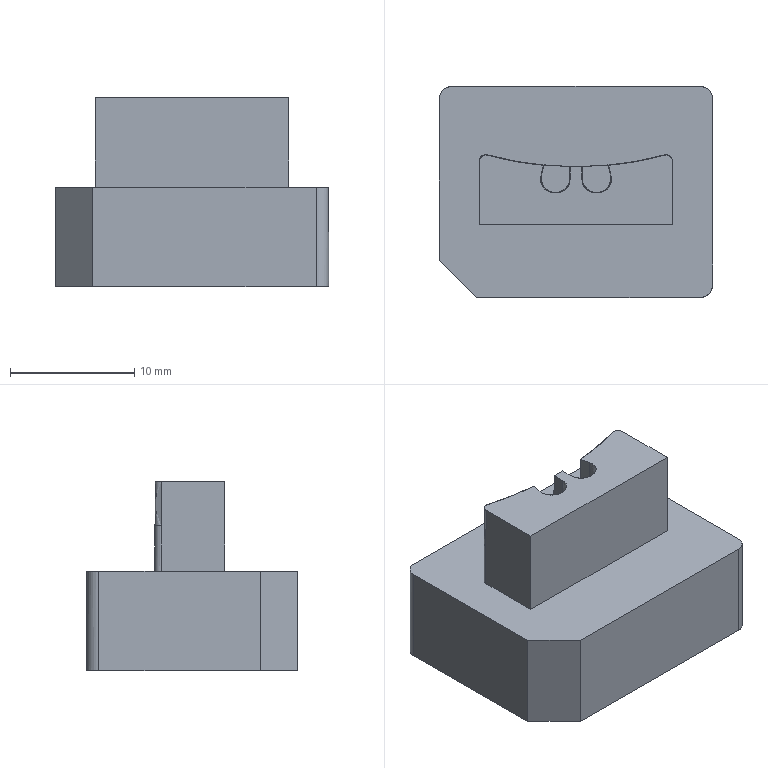NC program | PowerMill | posted by the shop | part box 22 x 17 x 15.232 mm
Lines 1 to 1558 of 87032:
%
G40 G49 G17 G80
( TOOL ID   D10C_1_1 )
( TOOL DIA. 10. TIP RAD 0 LENGTH 70.68 )
( Z = -.048 )
T1 M6
T15
G91 G28 Z0
G0 G90 G54
M08
S8000 M3
G0 X0 Y0 M8
G43 Z10.2 H1
X13.8 Y11.3
Z1.152
G1 Z-.048 F6000
X-13.8 F10000
Y5.65
X13.8
Y0
X-13.8
Y-5.65
X13.8
Y-11.3
X-13.8
X-18.8
G0 Z10.2
X.001 Y0
Z9.902
X-20.847 Y-7.452
Z.705
G1 Z-.495 F6000
X-20.319 F10000
G3 X-15.572 Y-2.705 I0 J4.748
G1 Y10.3
G2 X-14.572 Y11.3 I1. J0
G1 X14.573
G2 X15.573 Y10.3 I0 J-1.
G1 Y-10.3
G2 X14.573 Y-11.3 I-1. J0
G1 X-14.572
G2 X-15.572 Y-10.3 I0 J1.
G1 Y-2.705
X-13.073 Y-2.707
X-13.068 Y2.707
X-12.979 Y3.48
X-12.791 Y4.254
X-12.473 Y5.027
X-12.016 Y5.801
X-11.601 Y6.326
X-11.366 Y6.574
X-10.827 Y7.047
X-10.396 Y7.348
X-10.054 Y7.553
X-9.281 Y7.906
X-8.531 Y8.121
X-7.734 Y8.246
X-6.96 Y8.25
X-6.187 Y8.161
X-4.64 Y7.797
X-3.093 Y7.528
X-1.703 Y7.348
X-1.341 Y7.267
X-1.262 Y7.256
X-1.183 Y7.258
X-.773 Y7.299
X.774
X1.181 Y7.258
X1.26 Y7.256
X1.339 Y7.267
X1.702 Y7.348
X3.094 Y7.528
X4.641 Y7.797
X5.992 Y8.121
X6.961 Y8.25
X7.735 Y8.246
X8.508 Y8.126
X9.282 Y7.906
X10.055 Y7.553
X10.396 Y7.348
X10.828 Y7.046
X11.366 Y6.574
X11.602 Y6.326
X12.016 Y5.801
X12.375 Y5.216
X12.79 Y4.254
X12.978 Y3.48
X13.068 Y2.707
X13.073 Y-2.707
X13.004 Y-3.48
X12.817 Y-4.254
X12.498 Y-5.027
X12.375 Y-5.254
X12.017 Y-5.801
X11.602 Y-6.29
X11.308 Y-6.574
X10.828 Y-6.956
X10.179 Y-7.348
X9.282 Y-7.706
X8.508 Y-7.874
X7.735 Y-7.925
X-7.734
X-8.507 Y-7.874
X-9.281 Y-7.706
X-10.054 Y-7.409
X-10.827 Y-6.956
X-11.308 Y-6.574
X-11.601 Y-6.291
X-12.017 Y-5.801
X-12.374 Y-5.256
X-12.498 Y-5.027
X-12.817 Y-4.254
X-13.004 Y-3.48
X-13.073 Y-2.707
X-15.572 Y-2.705
G0 Z3.308
G1 X-20.847 Y-7.452
G0 Z.308
G1 Z-.892 F6000
X-20.319 F10000
G3 X-15.572 Y-2.705 I0 J4.748
G1 Y10.3
G2 X-14.572 Y11.3 I1. J0
G1 X14.573
G2 X15.573 Y10.3 I0 J-1.
G1 Y-10.3
G2 X14.573 Y-11.3 I-1. J0
G1 X-14.572
G2 X-15.572 Y-10.3 I0 J1.
G1 Y-2.705
X-13.073 Y-2.707
X-13.068 Y2.707
X-12.979 Y3.48
X-12.792 Y4.254
X-12.475 Y5.027
X-12.016 Y5.801
X-11.601 Y6.33
X-11.369 Y6.574
X-10.827 Y7.048
X-10.79 Y7.073
X-10.396 Y7.348
X-10.125 Y7.511
X-10.054 Y7.557
X-9.281 Y7.91
X-8.507 Y8.129
X-7.734 Y8.25
X-6.96 Y8.256
X-6.187 Y8.164
X-4.64 Y7.801
X-3.093 Y7.531
X-1.682 Y7.348
X-1.342 Y7.272
X-1.262 Y7.26
X-1.183 Y7.262
X-.773 Y7.303
X.774
X1.177 Y7.262
X1.26 Y7.261
X1.343 Y7.273
X1.547 Y7.321
X1.645 Y7.335
X1.702 Y7.348
X2.505 Y7.451
X3.094 Y7.531
X4.641 Y7.801
X5.976 Y8.121
X6.961 Y8.256
X7.735 Y8.25
X8.54 Y8.121
X9.282 Y7.909
X10.055 Y7.556
X10.12 Y7.514
X10.396 Y7.348
X10.791 Y7.072
X10.828 Y7.048
X11.37 Y6.574
X11.602 Y6.329
X12.016 Y5.801
X12.019 Y5.796
X12.375 Y5.216
X12.407 Y5.142
X12.475 Y5.027
X12.791 Y4.254
X12.979 Y3.48
X13.068 Y2.707
X13.073 Y-2.707
X13.004 Y-3.48
X12.817 Y-4.254
X12.498 Y-5.027
X12.375 Y-5.254
X12.017 Y-5.801
X11.602 Y-6.29
X11.308 Y-6.574
X10.828 Y-6.956
X10.179 Y-7.348
X9.282 Y-7.706
X8.508 Y-7.874
X7.735 Y-7.925
X-7.734
X-8.507 Y-7.874
X-9.281 Y-7.706
X-10.054 Y-7.409
X-10.827 Y-6.956
X-11.308 Y-6.574
X-11.601 Y-6.291
X-12.017 Y-5.801
X-12.374 Y-5.256
X-12.498 Y-5.027
X-12.817 Y-4.254
X-13.004 Y-3.48
X-13.073 Y-2.707
X-15.572 Y-2.705
G0 Z2.912
G1 X-20.847 Y-7.452
G0 Z-.088
G1 Z-1.288 F6000
X-20.319 F10000
G3 X-15.572 Y-2.705 I0 J4.748
G1 Y10.3
G2 X-14.572 Y11.3 I1. J0
G1 X14.573
G2 X15.573 Y10.3 I0 J-1.
G1 Y-10.3
G2 X14.573 Y-11.3 I-1. J0
G1 X-14.572
G2 X-15.572 Y-10.3 I0 J1.
G1 Y-2.705
X-13.073 Y-2.707
X-13.068 Y2.707
X-12.979 Y3.48
X-12.793 Y4.254
X-12.477 Y5.027
X-12.018 Y5.801
X-11.601 Y6.334
X-11.373 Y6.574
X-10.827 Y7.05
X-10.405 Y7.348
X-10.054 Y7.561
X-9.281 Y7.913
X-8.558 Y8.121
X-7.734 Y8.253
X-6.96 Y8.261
X-6.187 Y8.168
X-4.64 Y7.805
X-3.093 Y7.535
X-1.661 Y7.348
X-1.34 Y7.276
X-1.261 Y7.264
X-1.181 Y7.266
X-.773 Y7.307
X.774
X1.18 Y7.266
X1.26 Y7.264
X1.34 Y7.276
X1.66 Y7.348
X3.094 Y7.535
X4.641 Y7.806
X5.477 Y8.002
X5.976 Y8.121
X6.002 Y8.124
X6.188 Y8.168
X6.961 Y8.261
X7.735 Y8.253
X8.508 Y8.131
X9.282 Y7.912
X10.055 Y7.56
X10.405 Y7.348
X10.828 Y7.049
X11.373 Y6.574
X11.602 Y6.333
X12.018 Y5.801
X12.07 Y5.713
X12.375 Y5.216
X12.402 Y5.154
X12.477 Y5.027
X12.793 Y4.254
X12.98 Y3.48
X13.068 Y2.707
X13.073 Y-2.707
X13.004 Y-3.48
X12.817 Y-4.254
X12.498 Y-5.027
X12.375 Y-5.254
X12.017 Y-5.801
X11.602 Y-6.29
X11.308 Y-6.574
X10.828 Y-6.956
X10.179 Y-7.348
X9.282 Y-7.706
X8.508 Y-7.874
X7.735 Y-7.925
X-7.734
X-8.507 Y-7.874
X-9.281 Y-7.706
X-10.054 Y-7.409
X-10.827 Y-6.956
X-11.308 Y-6.574
X-11.601 Y-6.291
X-12.017 Y-5.801
X-12.374 Y-5.256
X-12.498 Y-5.027
X-12.817 Y-4.254
X-13.004 Y-3.48
X-13.073 Y-2.707
X-15.572 Y-2.705
G0 Z2.515
G1 X-20.847 Y-7.452
G0 Z-.485
G1 Z-1.685 F6000
X-20.319 F10000
G3 X-15.572 Y-2.705 I0 J4.748
G1 Y10.3
G2 X-14.572 Y11.3 I1. J0
G1 X14.573
G2 X15.573 Y10.3 I0 J-1.
G1 Y-10.3
G2 X14.573 Y-11.3 I-1. J0
G1 X-14.572
G2 X-15.572 Y-10.3 I0 J1.
G1 Y-2.705
X-13.073 Y-2.707
X-13.069 Y2.707
X-12.979 Y3.48
X-12.794 Y4.254
X-12.479 Y5.027
X-12.02 Y5.801
X-11.601 Y6.338
X-11.377 Y6.574
X-10.827 Y7.051
X-10.411 Y7.348
X-10.054 Y7.564
X-9.281 Y7.916
X-8.576 Y8.121
X-7.734 Y8.257
X-6.96 Y8.265
X-6.187 Y8.171
X-4.64 Y7.809
X-3.093 Y7.538
X-1.64 Y7.348
X-1.34 Y7.28
X-1.261 Y7.268
X-1.18 Y7.27
X-.773 Y7.311
X.774
X1.179 Y7.27
X1.259 Y7.268
X1.338 Y7.28
X1.64 Y7.348
X3.094 Y7.538
X4.641 Y7.809
X6.188 Y8.172
X6.961 Y8.265
X7.735 Y8.257
X8.508 Y8.135
X9.282 Y7.916
X10.055 Y7.564
X10.411 Y7.348
X10.828 Y7.051
X11.377 Y6.574
X11.602 Y6.336
X12.021 Y5.801
X12.144 Y5.593
X12.375 Y5.216
X12.397 Y5.166
X12.479 Y5.027
X12.794 Y4.254
X12.98 Y3.48
X13.069 Y2.707
X13.073 Y-2.707
X13.004 Y-3.48
X12.817 Y-4.254
X12.498 Y-5.027
X12.375 Y-5.254
X12.017 Y-5.801
X11.602 Y-6.29
X11.308 Y-6.574
X10.828 Y-6.956
X10.179 Y-7.348
X9.282 Y-7.706
X8.508 Y-7.874
X7.735 Y-7.925
X-7.734
X-8.507 Y-7.874
X-9.281 Y-7.706
X-10.054 Y-7.409
X-10.827 Y-6.956
X-11.308 Y-6.574
X-11.601 Y-6.291
X-12.017 Y-5.801
X-12.374 Y-5.256
X-12.498 Y-5.027
X-12.817 Y-4.254
X-13.004 Y-3.48
X-13.073 Y-2.707
X-15.572 Y-2.705
G0 Z2.118
G1 X-20.847 Y-7.452
G0 Z-.882
G1 Z-2.082 F6000
X-20.319 F10000
G3 X-15.572 Y-2.705 I0 J4.748
G1 Y10.3
G2 X-14.572 Y11.3 I1. J0
G1 X14.573
G2 X15.573 Y10.3 I0 J-1.
G1 Y-10.3
G2 X14.573 Y-11.3 I-1. J0
G1 X-14.572
G2 X-15.572 Y-10.3 I0 J1.
G1 Y-2.705
X-13.073 Y-2.707
X-13.069 Y2.707
X-12.979 Y3.48
X-12.795 Y4.254
X-12.481 Y5.027
X-12.024 Y5.801
X-11.601 Y6.341
X-11.38 Y6.574
X-10.827 Y7.053
X-10.416 Y7.348
X-10.054 Y7.568
X-9.281 Y7.919
X-8.593 Y8.121
X-7.734 Y8.261
X-6.96 Y8.268
X-6.187 Y8.175
X-4.64 Y7.813
X-3.093 Y7.542
X-1.619 Y7.348
X-1.341 Y7.284
X-1.261 Y7.273
X-1.18 Y7.274
X-.773 Y7.314
X.774
X1.178 Y7.274
X1.259 Y7.273
X1.338 Y7.284
X1.62 Y7.348
X3.094 Y7.542
X4.641 Y7.813
X6.188 Y8.175
X6.961 Y8.268
X7.735 Y8.261
X8.508 Y8.138
X9.282 Y7.919
X10.055 Y7.567
X10.417 Y7.348
X10.828 Y7.052
X11.38 Y6.574
X11.602 Y6.34
X12.023 Y5.801
X12.211 Y5.483
X12.375 Y5.216
X12.391 Y5.178
X12.481 Y5.027
X12.795 Y4.254
X12.98 Y3.48
X13.069 Y2.707
X13.073 Y-2.707
X13.004 Y-3.48
X12.817 Y-4.254
X12.498 Y-5.027
X12.375 Y-5.254
X12.017 Y-5.801
X11.602 Y-6.29
X11.308 Y-6.574
X10.828 Y-6.956
X10.179 Y-7.348
X9.282 Y-7.706
X8.508 Y-7.874
X7.735 Y-7.925
X-7.734
X-8.507 Y-7.874
X-9.281 Y-7.706
X-10.054 Y-7.409
X-10.827 Y-6.956
X-11.308 Y-6.574
X-11.601 Y-6.291
X-12.017 Y-5.801
X-12.374 Y-5.256
X-12.498 Y-5.027
X-12.817 Y-4.254
X-13.004 Y-3.48
X-13.073 Y-2.707
X-15.572 Y-2.705
G0 Z1.721
G1 X-20.847 Y-7.452
G0 Z-1.279
G1 Z-2.479 F6000
X-20.319 F10000
G3 X-15.572 Y-2.705 I0 J4.748
G1 Y10.3
G2 X-14.572 Y11.3 I1. J0
G1 X14.573
G2 X15.573 Y10.3 I0 J-1.
G1 Y-10.3
G2 X14.573 Y-11.3 I-1. J0
G1 X-14.572
G2 X-15.572 Y-10.3 I0 J1.
G1 Y-2.705
X-13.073 Y-2.707
X-13.069 Y2.707
X-12.98 Y3.48
X-12.796 Y4.254
X-12.482 Y5.027
X-12.027 Y5.801
X-11.601 Y6.345
X-11.384 Y6.574
X-10.827 Y7.056
X-10.424 Y7.348
X-10.054 Y7.571
X-9.281 Y7.923
X-8.611 Y8.121
X-7.734 Y8.264
X-6.96 Y8.272
X-6.187 Y8.179
X-4.64 Y7.816
X-4.337 Y7.759
X-3.687 Y7.645
X-1.546 Y7.337
X-1.342 Y7.289
X-1.261 Y7.277
X-1.179 Y7.278
X-.773 Y7.318
X.774
X1.178 Y7.278
X1.258 Y7.277
X1.338 Y7.288
X1.6 Y7.348
X3.094 Y7.545
X4.641 Y7.816
X6.188 Y8.179
X6.961 Y8.272
X7.735 Y8.264
X8.508 Y8.142
X9.282 Y7.922
X10.055 Y7.571
X10.424 Y7.348
X10.828 Y7.056
X11.384 Y6.574
X11.602 Y6.344
X12.027 Y5.801
X12.285 Y5.363
X12.375 Y5.216
X12.385 Y5.192
X12.482 Y5.027
X12.796 Y4.254
X12.981 Y3.48
X13.069 Y2.707
X13.073 Y-2.707
X13.004 Y-3.48
X12.817 Y-4.254
X12.498 Y-5.027
X12.375 Y-5.254
X12.017 Y-5.801
X11.602 Y-6.29
X11.308 Y-6.574
X10.828 Y-6.956
X10.179 Y-7.348
X9.282 Y-7.706
X8.508 Y-7.874
X7.735 Y-7.925
X-7.734
X-8.507 Y-7.874
X-9.281 Y-7.706
X-10.054 Y-7.409
X-10.827 Y-6.956
X-11.308 Y-6.574
X-11.601 Y-6.291
X-12.017 Y-5.801
X-12.374 Y-5.256
X-12.498 Y-5.027
X-12.817 Y-4.254
X-13.004 Y-3.48
X-13.073 Y-2.707
X-15.572 Y-2.705
G0 Z1.325
G1 X-20.847 Y-7.452
G0 Z-1.675
G1 Z-2.875 F6000
X-20.319 F10000
G3 X-15.572 Y-2.705 I0 J4.748
G1 Y10.3
G2 X-14.572 Y11.3 I1. J0
G1 X14.573
G2 X15.573 Y10.3 I0 J-1.
G1 Y-10.3
G2 X14.573 Y-11.3 I-1. J0
G1 X-14.572
G2 X-15.572 Y-10.3 I0 J1.
G1 Y-2.705
X-13.073 Y-2.707
X-13.069 Y2.707
X-12.981 Y3.48
X-12.798 Y4.254
X-12.484 Y5.027
X-12.031 Y5.801
X-11.601 Y6.348
X-11.388 Y6.574
X-10.827 Y7.061
X-10.431 Y7.348
X-10.054 Y7.575
X-9.281 Y7.926
X-8.629 Y8.121
X-7.734 Y8.268
X-6.96 Y8.275
X-6.187 Y8.182
X-4.64 Y7.82
X-4.037 Y7.707
X-3.802 Y7.666
X-1.546 Y7.341
X-1.34 Y7.293
X-1.259 Y7.281
X-1.177 Y7.282
X-.773 Y7.322
X.774
X1.178 Y7.282
X1.258 Y7.281
X1.338 Y7.292
X1.58 Y7.348
X3.094 Y7.549
X4.641 Y7.82
X6.188 Y8.182
X6.961 Y8.275
X7.735 Y8.268
X8.508 Y8.145
X9.282 Y7.926
X10.055 Y7.574
X10.431 Y7.348
X10.828 Y7.06
X11.388 Y6.574
X11.602 Y6.347
X12.031 Y5.801
X12.345 Y5.264
X12.375 Y5.216
X12.379 Y5.207
X12.484 Y5.027
X12.797 Y4.254
X12.981 Y3.48
X13.069 Y2.707
X13.073 Y-2.707
X13.004 Y-3.48
X12.817 Y-4.254
X12.498 Y-5.027
X12.375 Y-5.254
X12.017 Y-5.801
X11.602 Y-6.29
X11.308 Y-6.574
X10.828 Y-6.956
X10.179 Y-7.348
X9.282 Y-7.706
X8.508 Y-7.874
X7.735 Y-7.925
X-7.734
X-8.507 Y-7.874
X-9.281 Y-7.706
X-10.054 Y-7.409
X-10.827 Y-6.956
X-11.308 Y-6.574
X-11.601 Y-6.291
X-12.017 Y-5.801
X-12.374 Y-5.256
X-12.498 Y-5.027
X-12.817 Y-4.254
X-13.004 Y-3.48
X-13.073 Y-2.707
X-15.572 Y-2.705
G0 Z.928
G1 X-20.847 Y-7.452
G0 Z-2.072
G1 Z-3.272 F6000
X-20.319 F10000
G3 X-15.572 Y-2.705 I0 J4.748
G1 Y10.3
G2 X-14.572 Y11.3 I1. J0
G1 X14.573
G2 X15.573 Y10.3 I0 J-1.
G1 Y-10.3
G2 X14.573 Y-11.3 I-1. J0
G1 X-14.572
G2 X-15.572 Y-10.3 I0 J1.
G1 Y-2.705
X-13.073 Y-2.707
X-13.069 Y2.707
X-12.982 Y3.48
X-12.799 Y4.254
X-12.486 Y5.027
X-12.034 Y5.801
X-11.601 Y6.352
X-11.391 Y6.574
X-10.827 Y7.069
X-10.438 Y7.348
X-10.054 Y7.579
X-9.281 Y7.93
X-8.647 Y8.121
X-7.734 Y8.271
X-6.96 Y8.279
X-6.187 Y8.186
X-4.64 Y7.823
X-3.458 Y7.616
X-1.946 Y7.398
X-1.546 Y7.345
X-1.34 Y7.297
X-1.259 Y7.285
X-1.178 Y7.286
X-.773 Y7.325
X.774
X1.178 Y7.286
X1.258 Y7.285
X1.338 Y7.297
X1.56 Y7.348
X3.094 Y7.552
X4.641 Y7.823
X6.188 Y8.186
X6.961 Y8.279
X7.735 Y8.271
X8.508 Y8.151
X9.282 Y7.93
X10.055 Y7.578
X10.438 Y7.348
X10.828 Y7.068
X11.391 Y6.574
X11.602 Y6.351
X12.034 Y5.801
X12.486 Y5.027
X12.798 Y4.254
X12.981 Y3.48
X13.069 Y2.707
X13.073 Y-2.707
X13.004 Y-3.48
X12.817 Y-4.254
X12.498 Y-5.027
X12.375 Y-5.254
X12.017 Y-5.801
X11.602 Y-6.29
X11.308 Y-6.574
X10.828 Y-6.956
X10.179 Y-7.348
X9.282 Y-7.706
X8.508 Y-7.874
X7.735 Y-7.925
X-7.734
X-8.507 Y-7.874
X-9.281 Y-7.706
X-10.054 Y-7.409
X-10.827 Y-6.956
X-11.308 Y-6.574
X-11.601 Y-6.291
X-12.017 Y-5.801
X-12.374 Y-5.256
X-12.498 Y-5.027
X-12.817 Y-4.254
X-13.004 Y-3.48
X-13.073 Y-2.707
X-15.572 Y-2.705
G0 Z.531
G1 X-20.847 Y-7.452
G0 Z-2.469
G1 Z-3.669 F6000
X-20.319 F10000
G3 X-15.572 Y-2.705 I0 J4.748
G1 Y10.3
G2 X-14.572 Y11.3 I1. J0
G1 X14.573
G2 X15.573 Y10.3 I0 J-1.
G1 Y-10.3
G2 X14.573 Y-11.3 I-1. J0
G1 X-14.572
G2 X-15.572 Y-10.3 I0 J1.
G1 Y-2.705
X-13.073 Y-2.707
X-13.069 Y2.707
X-12.984 Y3.48
X-12.8 Y4.254
X-12.488 Y5.027
X-12.038 Y5.801
X-11.601 Y6.355
X-11.395 Y6.574
X-10.827 Y7.076
X-10.445 Y7.348
X-10.054 Y7.582
X-9.281 Y7.935
X-8.664 Y8.121
X-7.734 Y8.275
X-6.96 Y8.283
X-6.187 Y8.189
X-4.64 Y7.829
X-3.332 Y7.598
X-2.306 Y7.45
X-1.54 Y7.348
X-1.34 Y7.301
X-1.26 Y7.289
X-1.179 Y7.29
X-.773 Y7.329
X.774
X1.176 Y7.29
X1.257 Y7.289
X1.337 Y7.301
X1.547 Y7.349
X3.094 Y7.556
X4.641 Y7.829
X6.188 Y8.19
X6.961 Y8.283
X7.735 Y8.275
X8.508 Y8.157
X9.282 Y7.933
X10.055 Y7.582
X10.445 Y7.348
X10.828 Y7.076
X11.395 Y6.574
X11.602 Y6.354
X12.038 Y5.801
X12.488 Y5.027
X12.8 Y4.254
X12.982 Y3.48
X13.069 Y2.707
X13.073 Y-2.707
X13.004 Y-3.48
X12.817 Y-4.254
X12.498 Y-5.027
X12.375 Y-5.254
X12.017 Y-5.801
X11.602 Y-6.29
X11.308 Y-6.574
X10.828 Y-6.956
X10.179 Y-7.348
X9.282 Y-7.706
X8.508 Y-7.874
X7.735 Y-7.925
X-7.734
X-8.507 Y-7.874
X-9.281 Y-7.706
X-10.054 Y-7.409
X-10.827 Y-6.956
X-11.308 Y-6.574
X-11.601 Y-6.291
X-12.017 Y-5.801
X-12.374 Y-5.256
X-12.498 Y-5.027
X-12.817 Y-4.254
X-13.004 Y-3.48
X-13.073 Y-2.707
X-15.572 Y-2.705
G0 Z.134
G1 X-20.847 Y-7.452
G0 Z-2.866
G1 Z-4.066 F6000
X-20.319 F10000
G3 X-15.572 Y-2.705 I0 J4.748
G1 Y10.3
G2 X-14.572 Y11.3 I1. J0
G1 X14.573
G2 X15.573 Y10.3 I0 J-1.
G1 Y-10.3
G2 X14.573 Y-11.3 I-1. J0
G1 X-14.572
G2 X-15.572 Y-10.3 I0 J1.
G1 Y-2.705
X-13.073 Y-2.707
X-13.069 Y2.707
X-12.984 Y3.48
X-12.8 Y4.254
X-12.491 Y5.027
X-12.039 Y5.801
X-11.601 Y6.356
X-11.396 Y6.574
X-10.827 Y7.078
X-10.447 Y7.348
X-10.054 Y7.583
X-9.281 Y7.936
X-8.679 Y8.121
X-7.734 Y8.276
X-6.96 Y8.283
X-6.187 Y8.19
X-4.64 Y7.834
X-3.268 Y7.589
X-2.927 Y7.54
X-1.546 Y7.392
X.001 Y7.337
X1.547 Y7.392
X3.094 Y7.557
X4.641 Y7.834
X4.653 Y7.837
X6.188 Y8.19
X6.961 Y8.283
X7.735 Y8.276
X8.508 Y8.161
X9.282 Y7.936
X10.055 Y7.582
X10.447 Y7.348
X10.828 Y7.077
X11.396 Y6.574
X11.602 Y6.355
X12.039 Y5.801
X12.491 Y5.027
X12.8 Y4.254
X12.984 Y3.48
X13.069 Y2.707
X13.073 Y-2.707
X13.004 Y-3.48
X12.817 Y-4.254
X12.498 Y-5.027
X12.375 Y-5.254
X12.017 Y-5.801
X11.602 Y-6.29
X11.308 Y-6.574
X10.828 Y-6.956
X10.179 Y-7.348
X9.282 Y-7.706
X8.508 Y-7.874
X7.735 Y-7.925
X-7.734
X-8.507 Y-7.874
X-9.281 Y-7.706
X-10.054 Y-7.409
X-10.827 Y-6.956
X-11.308 Y-6.574
X-11.601 Y-6.291
X-12.017 Y-5.801
X-12.374 Y-5.256
X-12.498 Y-5.027
X-12.817 Y-4.254
X-13.004 Y-3.48
X-13.073 Y-2.707
X-15.572 Y-2.705
G0 Z-.263
G1 X-20.847 Y-7.452
G0 Z-3.263
G1 Z-4.463 F6000
X-20.319 F10000
G3 X-15.572 Y-2.705 I0 J4.748
G1 Y10.3
G2 X-14.572 Y11.3 I1. J0
G1 X14.573
G2 X15.573 Y10.3 I0 J-1.
G1 Y-10.3
G2 X14.573 Y-11.3 I-1. J0
G1 X-14.572
G2 X-15.572 Y-10.3 I0 J1.
G1 Y-2.705
X-13.073 Y-2.707
X-13.069 Y2.707
X-12.984 Y3.48
X-12.8 Y4.254
X-12.491 Y5.027
X-12.039 Y5.801
X-11.601 Y6.356
X-11.396 Y6.574
X-10.827 Y7.078
X-10.447 Y7.348
X-10.054 Y7.583
X-9.281 Y7.936
X-8.679 Y8.121
X-7.734 Y8.276
X-6.96 Y8.283
X-6.187 Y8.19
X-4.64 Y7.834
X-3.266 Y7.588
X-2.929 Y7.54
X-1.546 Y7.392
X.001 Y7.337
X1.547 Y7.392
X3.094 Y7.558
X4.641 Y7.834
X4.653 Y7.837
X6.188 Y8.19
X6.961 Y8.283
X7.735 Y8.276
X8.508 Y8.161
X9.282 Y7.936
X10.055 Y7.582
X10.447 Y7.348
X10.828 Y7.077
X11.396 Y6.574
X11.602 Y6.355
X12.039 Y5.801
X12.491 Y5.027
X12.8 Y4.254
X12.984 Y3.48
X13.069 Y2.707
X13.073 Y-2.707
X13.004 Y-3.48
X12.817 Y-4.254
X12.498 Y-5.027
X12.375 Y-5.254
X12.017 Y-5.801
X11.602 Y-6.29
X11.308 Y-6.574
X10.828 Y-6.956
X10.179 Y-7.348
X9.282 Y-7.706
X8.508 Y-7.874
X7.735 Y-7.925
X-7.734
X-8.507 Y-7.874
X-9.281 Y-7.706
X-10.054 Y-7.409
X-10.827 Y-6.956
X-11.308 Y-6.574
X-11.601 Y-6.291
X-12.017 Y-5.801
X-12.374 Y-5.256
X-12.498 Y-5.027
X-12.817 Y-4.254
X-13.004 Y-3.48
X-13.073 Y-2.707
X-15.572 Y-2.705
G0 Z-.659
G1 X-20.847 Y-7.452
G0 Z-3.659
G1 Z-4.859 F6000
X-20.319 F10000
G3 X-15.572 Y-2.705 I0 J4.748
G1 Y10.3
G2 X-14.572 Y11.3 I1. J0
G1 X14.573
G2 X15.573 Y10.3 I0 J-1.
G1 Y-10.3
G2 X14.573 Y-11.3 I-1. J0
G1 X-14.572
G2 X-15.572 Y-10.3 I0 J1.
G1 Y-2.705
X-13.073 Y-2.707
X-13.069 Y2.707
X-12.984 Y3.48
X-12.8 Y4.254
X-12.491 Y5.027
X-12.039 Y5.801
X-11.601 Y6.356
X-11.396 Y6.574
X-10.827 Y7.078
X-10.447 Y7.348
X-10.054 Y7.583
X-9.281 Y7.936
X-8.679 Y8.121
X-7.734 Y8.276
X-6.96 Y8.283
X-6.187 Y8.19
X-4.64 Y7.834
X-3.264 Y7.588
X-2.93 Y7.54
X-1.546 Y7.392
X.001 Y7.337
X1.547 Y7.392
X3.094 Y7.558
X4.641 Y7.834
X4.653 Y7.837
X6.188 Y8.19
X6.961 Y8.284
X7.735 Y8.276
X8.508 Y8.161
X9.282 Y7.936
X10.055 Y7.582
X10.447 Y7.348
X10.828 Y7.077
X11.396 Y6.574
X11.602 Y6.355
X12.039 Y5.801
X12.491 Y5.027
X12.8 Y4.254
X12.984 Y3.48
X13.069 Y2.707
X13.073 Y-2.707
X13.004 Y-3.48
X12.817 Y-4.254
X12.498 Y-5.027
X12.375 Y-5.254
X12.017 Y-5.801
X11.602 Y-6.29
X11.308 Y-6.574
X10.828 Y-6.956
X10.179 Y-7.348
X9.282 Y-7.706
X8.508 Y-7.874
X7.735 Y-7.925
X-7.734
X-8.507 Y-7.874
X-9.281 Y-7.706
X-10.054 Y-7.409
X-10.827 Y-6.956
X-11.308 Y-6.574
X-11.601 Y-6.291
X-12.017 Y-5.801
X-12.374 Y-5.256
X-12.498 Y-5.027
X-12.817 Y-4.254
X-13.004 Y-3.48
X-13.073 Y-2.707
X-15.572 Y-2.705
G0 Z-1.056
G1 X-20.847 Y-7.452
G0 Z-4.056
G1 Z-5.256 F6000
X-20.319 F10000
G3 X-15.572 Y-2.705 I0 J4.748
G1 Y10.3
G2 X-14.572 Y11.3 I1. J0
G1 X14.573
G2 X15.573 Y10.3 I0 J-1.
G1 Y-10.3
G2 X14.573 Y-11.3 I-1. J0
G1 X-14.572
G2 X-15.572 Y-10.3 I0 J1.
G1 Y-2.705
X-13.073 Y-2.707
X-13.069 Y2.707
X-12.984 Y3.48
X-12.8 Y4.254
X-12.491 Y5.027
X-12.039 Y5.801
X-11.601 Y6.356
X-11.396 Y6.574
X-10.827 Y7.078
X-10.447 Y7.348
X-10.054 Y7.583
X-9.281 Y7.936
X-8.679 Y8.121
X-7.734 Y8.276
X-6.96 Y8.283
X-6.187 Y8.19
X-4.64 Y7.834
X-3.263 Y7.588
X-2.932 Y7.54
X-1.546 Y7.392
X.001 Y7.337
X1.547 Y7.392
X3.094 Y7.558
X4.641 Y7.834
X4.653 Y7.837
X6.188 Y8.19
X6.961 Y8.284
X7.735 Y8.276
X8.508 Y8.161
X9.282 Y7.936
X10.055 Y7.582
X10.447 Y7.348
X10.828 Y7.077
X11.396 Y6.574
X11.602 Y6.355
X12.039 Y5.801
X12.491 Y5.027
X12.8 Y4.254
X12.984 Y3.48
X13.069 Y2.707
X13.073 Y-2.707
X13.004 Y-3.48
X12.817 Y-4.254
X12.498 Y-5.027
X12.375 Y-5.254
X12.017 Y-5.801
X11.602 Y-6.29
X11.308 Y-6.574
X10.828 Y-6.956
X10.179 Y-7.348
X9.282 Y-7.706
X8.508 Y-7.874
X7.735 Y-7.925
X-7.734
X-8.507 Y-7.874
X-9.281 Y-7.706
X-10.054 Y-7.409
X-10.827 Y-6.956
X-11.308 Y-6.574
X-11.601 Y-6.291
X-12.017 Y-5.801
X-12.374 Y-5.256
X-12.498 Y-5.027
X-12.817 Y-4.254
X-13.004 Y-3.48
X-13.073 Y-2.707
X-15.572 Y-2.705
G0 Z-1.453
G1 X-20.847 Y-7.452
G0 Z-4.453
G1 Z-5.653 F6000
X-20.319 F10000
G3 X-15.572 Y-2.705 I0 J4.748
G1 Y10.3
G2 X-14.572 Y11.3 I1. J0
G1 X14.573
G2 X15.573 Y10.3 I0 J-1.
G1 Y-10.3
G2 X14.573 Y-11.3 I-1. J0
G1 X-14.572
G2 X-15.572 Y-10.3 I0 J1.
G1 Y-2.705
X-13.073 Y-2.707
X-13.069 Y2.707
X-12.984 Y3.48
X-12.8 Y4.254
X-12.491 Y5.027
X-12.039 Y5.801
X-11.601 Y6.356
X-11.396 Y6.574
X-10.827 Y7.078
X-10.447 Y7.348
X-10.054 Y7.583
X-9.281 Y7.936
X-8.679 Y8.121
X-7.734 Y8.276
X-6.96 Y8.283
X-6.187 Y8.19
X-4.64 Y7.834
X-3.261 Y7.587
X-2.934 Y7.54
X-1.546 Y7.392
X.001 Y7.337
X1.547 Y7.392
X3.094 Y7.558
X4.641 Y7.834
X4.653 Y7.837
X6.188 Y8.19
X6.961 Y8.284
X7.735 Y8.276
X8.508 Y8.161
X9.282 Y7.936
X10.055 Y7.582
X10.447 Y7.348
X10.828 Y7.077
X11.396 Y6.574
X11.602 Y6.355
X12.039 Y5.801
X12.491 Y5.027
X12.8 Y4.254
X12.984 Y3.48
X13.069 Y2.707
X13.073 Y-2.707
X13.004 Y-3.48
X12.817 Y-4.254
X12.498 Y-5.027
X12.375 Y-5.254
X12.017 Y-5.801
X11.602 Y-6.29
X11.308 Y-6.574
X10.828 Y-6.956
X10.179 Y-7.348
X9.282 Y-7.706
X8.508 Y-7.874
X7.735 Y-7.925
X-7.734
X-8.507 Y-7.874
X-9.281 Y-7.706
X-10.054 Y-7.409
X-10.827 Y-6.956
X-11.308 Y-6.574
X-11.601 Y-6.291
X-12.017 Y-5.801
X-12.374 Y-5.256
X-12.498 Y-5.027
X-12.817 Y-4.254
X-13.004 Y-3.48
X-13.073 Y-2.707
X-15.572 Y-2.705
G0 Z-1.85
G1 X-20.847 Y-7.452
G0 Z-4.85
G1 Z-6.05 F6000
X-20.319 F10000
G3 X-15.572 Y-2.705 I0 J4.748
G1 Y10.3
G2 X-14.572 Y11.3 I1. J0
G1 X14.573
G2 X15.573 Y10.3 I0 J-1.
G1 Y-10.3
G2 X14.573 Y-11.3 I-1. J0
G1 X-14.572
G2 X-15.572 Y-10.3 I0 J1.
G1 Y-2.705
X-13.073 Y-2.707
X-13.069 Y2.707
X-12.984 Y3.48
X-12.8 Y4.254
X-12.491 Y5.027
X-12.039 Y5.801
X-11.601 Y6.356
X-11.396 Y6.574
X-10.827 Y7.078
X-10.447 Y7.348
X-10.054 Y7.583
X-9.281 Y7.936
X-8.679 Y8.121
X-7.734 Y8.276
X-6.96 Y8.283
X-6.187 Y8.19
X-4.64 Y7.834
X-3.259 Y7.587
X-2.935 Y7.54
X-1.546 Y7.392
X.001 Y7.337
X1.547 Y7.392
X3.094 Y7.558
X4.641 Y7.834
X4.653 Y7.837
X6.188 Y8.191
X6.961 Y8.284
X7.735 Y8.276
X8.508 Y8.162
X9.282 Y7.936
X10.055 Y7.583
X10.447 Y7.348
X10.828 Y7.077
X11.396 Y6.574
X11.602 Y6.355
X12.039 Y5.801
X12.491 Y5.027
X12.8 Y4.254
X12.984 Y3.48
X13.069 Y2.707
X13.073 Y-2.707
X13.004 Y-3.48
X12.817 Y-4.254
X12.498 Y-5.027
X12.375 Y-5.254
X12.017 Y-5.801
X11.602 Y-6.29
X11.308 Y-6.574
X10.828 Y-6.956
X10.179 Y-7.348
X9.282 Y-7.706
X8.508 Y-7.874
X7.735 Y-7.925
X-7.734
X-8.507 Y-7.874
X-9.281 Y-7.706
X-10.054 Y-7.409
X-10.827 Y-6.956
X-11.308 Y-6.574
X-11.601 Y-6.291
X-12.017 Y-5.801
X-12.374 Y-5.256
X-12.498 Y-5.027
X-12.817 Y-4.254
X-13.004 Y-3.48
X-13.073 Y-2.707
X-15.572 Y-2.705
G0 Z-2.246
G1 X-20.847 Y-7.452
G0 Z-5.246
G1 Z-6.446 F6000
X-20.319 F10000
G3 X-15.572 Y-2.705 I0 J4.748
G1 Y10.3
G2 X-14.572 Y11.3 I1. J0
G1 X14.573
G2 X15.573 Y10.3 I0 J-1.
G1 Y-10.3
G2 X14.573 Y-11.3 I-1. J0
G1 X-14.572
G2 X-15.572 Y-10.3 I0 J1.
G1 Y-2.705
X-13.073 Y-2.707
X-13.069 Y2.707
X-12.984 Y3.48
X-12.8 Y4.254
X-12.491 Y5.027
X-12.039 Y5.801
X-11.601 Y6.356
X-11.396 Y6.574
X-10.827 Y7.078
X-10.447 Y7.348
X-10.054 Y7.583
X-9.281 Y7.936
X-8.679 Y8.121
X-7.734 Y8.276
X-6.96 Y8.283
X-6.187 Y8.19
X-4.64 Y7.834
X-3.258 Y7.587
X-2.937 Y7.541
X-1.546 Y7.392
X.001 Y7.337
X1.547 Y7.392
X3.094 Y7.558
X4.641 Y7.834
X4.653 Y7.837
X6.188 Y8.191
X6.961 Y8.284
X7.735 Y8.276
X8.508 Y8.162
X9.282 Y7.936
X10.055 Y7.583
X10.447 Y7.348
X10.828 Y7.077
X11.396 Y6.574
X11.602 Y6.355
X12.039 Y5.801
X12.491 Y5.027
X12.8 Y4.254
X12.984 Y3.48
X13.069 Y2.707
X13.073 Y-2.707
X13.004 Y-3.48
X12.817 Y-4.254
X12.498 Y-5.027
X12.375 Y-5.254
X12.017 Y-5.801
X11.602 Y-6.29
X11.308 Y-6.574
X10.828 Y-6.956
X10.179 Y-7.348
X9.282 Y-7.706
X8.508 Y-7.874
X7.735 Y-7.925
X-7.734
X-8.507 Y-7.874
X-9.281 Y-7.706
X-10.054 Y-7.409
X-10.827 Y-6.956
X-11.308 Y-6.574
X-11.601 Y-6.291
X-12.017 Y-5.801
X-12.374 Y-5.256
X-12.498 Y-5.027
X-12.817 Y-4.254
X-13.004 Y-3.48
X-13.073 Y-2.707
X-15.572 Y-2.705
G0 Z-2.643
G1 X-20.847 Y-7.452
G0 Z-5.643
G1 Z-6.843 F6000
X-20.319 F10000
G3 X-15.572 Y-2.705 I0 J4.748
G1 Y10.3
G2 X-14.572 Y11.3 I1. J0
G1 X14.573
G2 X15.573 Y10.3 I0 J-1.
G1 Y-10.3
G2 X14.573 Y-11.3 I-1. J0
G1 X-14.572
G2 X-15.572 Y-10.3 I0 J1.
G1 Y-2.705
X-13.073 Y-2.707
X-13.069 Y2.707
X-12.984 Y3.48
X-12.8 Y4.254
X-12.491 Y5.027
X-12.039 Y5.801
X-11.601 Y6.356
X-11.396 Y6.574
X-10.827 Y7.078
X-10.447 Y7.348
X-10.054 Y7.583
X-9.281 Y7.936
X-8.679 Y8.121
X-7.734 Y8.276
X-6.96 Y8.283
X-6.187 Y8.19
X-4.64 Y7.834
X-3.256 Y7.586
X-2.939 Y7.541
X-1.546 Y7.392
X.001 Y7.337
X1.547 Y7.392
X3.094 Y7.558
X4.641 Y7.834
X4.653 Y7.837
X6.188 Y8.191
X6.961 Y8.284
X7.735 Y8.276
X8.508 Y8.162
X9.282 Y7.936
X10.055 Y7.583
X10.447 Y7.348
X10.828 Y7.077
X11.396 Y6.574
X11.602 Y6.355
X12.039 Y5.801
X12.491 Y5.027
X12.8 Y4.254
X12.984 Y3.48
X13.069 Y2.707
X13.073 Y-2.707
X13.004 Y-3.48
X12.817 Y-4.254
X12.498 Y-5.027
X12.375 Y-5.254
X12.017 Y-5.801
X11.602 Y-6.29
X11.308 Y-6.574
X10.828 Y-6.956
X10.179 Y-7.348
X9.282 Y-7.706
X8.508 Y-7.874
X7.735 Y-7.925
X-7.734
X-8.507 Y-7.874
X-9.281 Y-7.706
X-10.054 Y-7.409
X-10.827 Y-6.956
X-11.308 Y-6.574
X-11.601 Y-6.291
X-12.017 Y-5.801
X-12.374 Y-5.256
X-12.498 Y-5.027
X-12.817 Y-4.254
X-13.004 Y-3.48
X-13.073 Y-2.707
X-15.572 Y-2.705
G0 Z-3.04
G1 X-20.847 Y-7.452
G0 Z-6.04
G1 Z-7.24 F6000
X-20.319 F10000
G3 X-15.572 Y-2.705 I0 J4.748
G1 Y10.3
G2 X-14.572 Y11.3 I1. J0
G1 X14.573
G2 X15.573 Y10.3 I0 J-1.
G1 Y-10.3
G2 X14.573 Y-11.3 I-1. J0
G1 X-14.572
G2 X-15.572 Y-10.3 I0 J1.
G1 Y-2.705
X-13.073 Y-2.707
X-13.069 Y2.707
X-12.984 Y3.48
X-12.8 Y4.254
X-12.491 Y5.027
X-12.039 Y5.801
X-11.601 Y6.356
X-11.396 Y6.574
X-10.827 Y7.078
X-10.447 Y7.348
X-10.054 Y7.583
X-9.281 Y7.936
X-8.679 Y8.121
X-7.734 Y8.276
X-6.96 Y8.283
X-6.187 Y8.19
X-4.64 Y7.834
X-3.254 Y7.586
X-2.94 Y7.541
X-1.546 Y7.392
X.001 Y7.337
X1.547 Y7.392
X3.094 Y7.558
X4.641 Y7.834
X4.653 Y7.837
X6.188 Y8.191
X6.961 Y8.284
X7.735 Y8.276
X8.508 Y8.162
X9.282 Y7.936
X10.055 Y7.583
X10.447 Y7.348
X10.828 Y7.077
X11.396 Y6.574
X11.602 Y6.355
X12.039 Y5.801
X12.491 Y5.027
X12.8 Y4.254
X12.984 Y3.48
X13.069 Y2.707
X13.073 Y-2.707
X13.004 Y-3.48
X12.817 Y-4.254